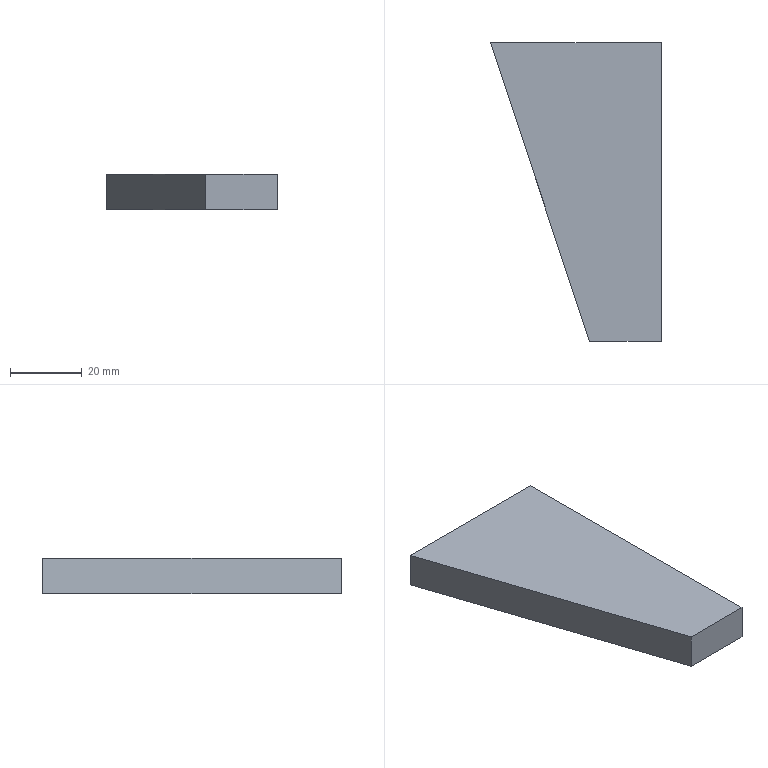Part | STEP file | 02-Reinforcing rib 13 | 1 solid | 6 faces | box 47.5 x 83 x 10 mm | volume 28013 mm3 | plane 6
STEP:
#1=CARTESIAN_POINT('',(0.,0.,0.));
#2=DIRECTION('',(0.,0.,1.));
#3=DIRECTION('',(1.,0.,0.));
#4=AXIS2_PLACEMENT_3D('',#1,#2,#3);
#5=CARTESIAN_POINT('',(0.,-83.,0.));
#6=VERTEX_POINT('',#5);
#7=CARTESIAN_POINT('',(0.,0.,0.));
#8=VERTEX_POINT('',#7);
#9=CARTESIAN_POINT('',(0.,0.,0.));
#10=DIRECTION('',(0.,1.,0.));
#11=VECTOR('',#10,1.);
#12=LINE('',#9,#11);
#13=CARTESIAN_POINT('',(0.,0.,10.));
#14=DIRECTION('',(-1.,0.,0.));
#15=DIRECTION('',(0.,-1.,0.));
#16=AXIS2_PLACEMENT_3D('',#13,#14,#15);
#17=PLANE('',#16);
#18=CARTESIAN_POINT('',(0.,-10.));
#19=DIRECTION('',(-1.,0.));
#20=VECTOR('',#19,1.);
#21=LINE('',#18,#20);
#22=(GEOMETRIC_REPRESENTATION_CONTEXT(2)PARAMETRIC_REPRESENTATION_CONTEXT()REPRESENTATION_CONTEXT('',''));
#23=DEFINITIONAL_REPRESENTATION('',(#21),#22);
#24=PCURVE('',#17,#23);
#25=CARTESIAN_POINT('',(0.,0.,0.));
#26=DIRECTION('',(0.,0.,-1.));
#27=DIRECTION('',(-1.,0.,0.));
#28=AXIS2_PLACEMENT_3D('',#25,#26,#27);
#29=PLANE('',#28);
#30=CARTESIAN_POINT('',(0.,0.));
#31=DIRECTION('',(0.,1.));
#32=VECTOR('',#31,1.);
#33=LINE('',#30,#32);
#34=(GEOMETRIC_REPRESENTATION_CONTEXT(2)PARAMETRIC_REPRESENTATION_CONTEXT()REPRESENTATION_CONTEXT('',''));
#35=DEFINITIONAL_REPRESENTATION('',(#33),#34);
#36=PCURVE('',#29,#35);
#37=SURFACE_CURVE('',#12,(#24,#36),.PCURVE_S1.);
#38=EDGE_CURVE('',#6,#8,#37,.T.);
#39=ORIENTED_EDGE('',*,*,#38,.T.);
#40=CARTESIAN_POINT('',(0.,0.,10.));
#41=VERTEX_POINT('',#40);
#42=CARTESIAN_POINT('',(0.,0.,10.));
#43=DIRECTION('',(0.,0.,-1.));
#44=VECTOR('',#43,1.);
#45=LINE('',#42,#44);
#46=CARTESIAN_POINT('',(0.,0.));
#47=DIRECTION('',(0.,-1.));
#48=VECTOR('',#47,1.);
#49=LINE('',#46,#48);
#50=(GEOMETRIC_REPRESENTATION_CONTEXT(2)PARAMETRIC_REPRESENTATION_CONTEXT()REPRESENTATION_CONTEXT('',''));
#51=DEFINITIONAL_REPRESENTATION('',(#49),#50);
#52=PCURVE('',#17,#51);
#53=CARTESIAN_POINT('',(0.,0.,10.));
#54=DIRECTION('',(0.,-1.,0.));
#55=DIRECTION('',(1.,0.,0.));
#56=AXIS2_PLACEMENT_3D('',#53,#54,#55);
#57=PLANE('',#56);
#58=CARTESIAN_POINT('',(0.,0.));
#59=DIRECTION('',(0.,-1.));
#60=VECTOR('',#59,1.);
#61=LINE('',#58,#60);
#62=(GEOMETRIC_REPRESENTATION_CONTEXT(2)PARAMETRIC_REPRESENTATION_CONTEXT()REPRESENTATION_CONTEXT('',''));
#63=DEFINITIONAL_REPRESENTATION('',(#61),#62);
#64=PCURVE('',#57,#63);
#65=SURFACE_CURVE('',#45,(#52,#64),.PCURVE_S1.);
#66=EDGE_CURVE('',#41,#8,#65,.T.);
#67=ORIENTED_EDGE('',*,*,#66,.F.);
#68=CARTESIAN_POINT('',(0.,-83.,10.));
#69=VERTEX_POINT('',#68);
#70=CARTESIAN_POINT('',(0.,0.,10.));
#71=DIRECTION('',(0.,1.,0.));
#72=VECTOR('',#71,1.);
#73=LINE('',#70,#72);
#74=CARTESIAN_POINT('',(0.,0.));
#75=DIRECTION('',(-1.,0.));
#76=VECTOR('',#75,1.);
#77=LINE('',#74,#76);
#78=(GEOMETRIC_REPRESENTATION_CONTEXT(2)PARAMETRIC_REPRESENTATION_CONTEXT()REPRESENTATION_CONTEXT('',''));
#79=DEFINITIONAL_REPRESENTATION('',(#77),#78);
#80=PCURVE('',#17,#79);
#81=CARTESIAN_POINT('',(0.,0.,10.));
#82=DIRECTION('',(0.,0.,-1.));
#83=DIRECTION('',(-1.,0.,0.));
#84=AXIS2_PLACEMENT_3D('',#81,#82,#83);
#85=PLANE('',#84);
#86=CARTESIAN_POINT('',(0.,0.));
#87=DIRECTION('',(0.,1.));
#88=VECTOR('',#87,1.);
#89=LINE('',#86,#88);
#90=(GEOMETRIC_REPRESENTATION_CONTEXT(2)PARAMETRIC_REPRESENTATION_CONTEXT()REPRESENTATION_CONTEXT('',''));
#91=DEFINITIONAL_REPRESENTATION('',(#89),#90);
#92=PCURVE('',#85,#91);
#93=SURFACE_CURVE('',#73,(#80,#92),.PCURVE_S1.);
#94=EDGE_CURVE('',#69,#41,#93,.T.);
#95=ORIENTED_EDGE('',*,*,#94,.F.);
#96=CARTESIAN_POINT('',(0.,-83.,10.));
#97=DIRECTION('',(0.,0.,-1.));
#98=VECTOR('',#97,1.);
#99=LINE('',#96,#98);
#100=CARTESIAN_POINT('',(83.,0.));
#101=DIRECTION('',(0.,-1.));
#102=VECTOR('',#101,1.);
#103=LINE('',#100,#102);
#104=(GEOMETRIC_REPRESENTATION_CONTEXT(2)PARAMETRIC_REPRESENTATION_CONTEXT()REPRESENTATION_CONTEXT('',''));
#105=DEFINITIONAL_REPRESENTATION('',(#103),#104);
#106=PCURVE('',#17,#105);
#107=CARTESIAN_POINT('',(0.,-83.,10.));
#108=DIRECTION('',(0.,1.,0.));
#109=DIRECTION('',(0.,0.,1.));
#110=AXIS2_PLACEMENT_3D('',#107,#108,#109);
#111=PLANE('',#110);
#112=CARTESIAN_POINT('',(0.,0.));
#113=DIRECTION('',(-1.,0.));
#114=VECTOR('',#113,1.);
#115=LINE('',#112,#114);
#116=(GEOMETRIC_REPRESENTATION_CONTEXT(2)PARAMETRIC_REPRESENTATION_CONTEXT()REPRESENTATION_CONTEXT('',''));
#117=DEFINITIONAL_REPRESENTATION('',(#115),#116);
#118=PCURVE('',#111,#117);
#119=SURFACE_CURVE('',#99,(#106,#118),.PCURVE_S1.);
#120=EDGE_CURVE('',#69,#6,#119,.T.);
#121=ORIENTED_EDGE('',*,*,#120,.T.);
#122=EDGE_LOOP('',(#39,#67,#95,#121));
#123=FACE_BOUND('',#122,.T.);
#124=ADVANCED_FACE('',(#123),#17,.F.);
#125=CARTESIAN_POINT('',(-47.5,0.,0.));
#126=VERTEX_POINT('',#125);
#127=CARTESIAN_POINT('',(0.,0.,0.));
#128=DIRECTION('',(-1.,0.,0.));
#129=VECTOR('',#128,1.);
#130=LINE('',#127,#129);
#131=CARTESIAN_POINT('',(0.,-10.));
#132=DIRECTION('',(-1.,0.));
#133=VECTOR('',#132,1.);
#134=LINE('',#131,#133);
#135=(GEOMETRIC_REPRESENTATION_CONTEXT(2)PARAMETRIC_REPRESENTATION_CONTEXT()REPRESENTATION_CONTEXT('',''));
#136=DEFINITIONAL_REPRESENTATION('',(#134),#135);
#137=PCURVE('',#57,#136);
#138=CARTESIAN_POINT('',(0.,0.));
#139=DIRECTION('',(1.,0.));
#140=VECTOR('',#139,1.);
#141=LINE('',#138,#140);
#142=(GEOMETRIC_REPRESENTATION_CONTEXT(2)PARAMETRIC_REPRESENTATION_CONTEXT()REPRESENTATION_CONTEXT('',''));
#143=DEFINITIONAL_REPRESENTATION('',(#141),#142);
#144=PCURVE('',#29,#143);
#145=SURFACE_CURVE('',#130,(#137,#144),.PCURVE_S1.);
#146=EDGE_CURVE('',#8,#126,#145,.T.);
#147=ORIENTED_EDGE('',*,*,#146,.T.);
#148=CARTESIAN_POINT('',(-47.5,0.,10.));
#149=VERTEX_POINT('',#148);
#150=CARTESIAN_POINT('',(-47.5,0.,10.));
#151=DIRECTION('',(0.,0.,-1.));
#152=VECTOR('',#151,1.);
#153=LINE('',#150,#152);
#154=CARTESIAN_POINT('',(-47.5,0.));
#155=DIRECTION('',(0.,-1.));
#156=VECTOR('',#155,1.);
#157=LINE('',#154,#156);
#158=(GEOMETRIC_REPRESENTATION_CONTEXT(2)PARAMETRIC_REPRESENTATION_CONTEXT()REPRESENTATION_CONTEXT('',''));
#159=DEFINITIONAL_REPRESENTATION('',(#157),#158);
#160=PCURVE('',#57,#159);
#161=CARTESIAN_POINT('',(-20.,-83.,10.));
#162=DIRECTION('',(0.9493,0.3145,0.));
#163=DIRECTION('',(-0.3145,0.9493,0.));
#164=AXIS2_PLACEMENT_3D('',#161,#162,#163);
#165=PLANE('',#164);
#166=CARTESIAN_POINT('',(87.437,0.));
#167=DIRECTION('',(0.,-1.));
#168=VECTOR('',#167,1.);
#169=LINE('',#166,#168);
#170=(GEOMETRIC_REPRESENTATION_CONTEXT(2)PARAMETRIC_REPRESENTATION_CONTEXT()REPRESENTATION_CONTEXT('',''));
#171=DEFINITIONAL_REPRESENTATION('',(#169),#170);
#172=PCURVE('',#165,#171);
#173=SURFACE_CURVE('',#153,(#160,#172),.PCURVE_S1.);
#174=EDGE_CURVE('',#149,#126,#173,.T.);
#175=ORIENTED_EDGE('',*,*,#174,.F.);
#176=CARTESIAN_POINT('',(0.,0.,10.));
#177=DIRECTION('',(-1.,0.,0.));
#178=VECTOR('',#177,1.);
#179=LINE('',#176,#178);
#180=CARTESIAN_POINT('',(0.,0.));
#181=DIRECTION('',(-1.,0.));
#182=VECTOR('',#181,1.);
#183=LINE('',#180,#182);
#184=(GEOMETRIC_REPRESENTATION_CONTEXT(2)PARAMETRIC_REPRESENTATION_CONTEXT()REPRESENTATION_CONTEXT('',''));
#185=DEFINITIONAL_REPRESENTATION('',(#183),#184);
#186=PCURVE('',#57,#185);
#187=CARTESIAN_POINT('',(0.,0.));
#188=DIRECTION('',(1.,0.));
#189=VECTOR('',#188,1.);
#190=LINE('',#187,#189);
#191=(GEOMETRIC_REPRESENTATION_CONTEXT(2)PARAMETRIC_REPRESENTATION_CONTEXT()REPRESENTATION_CONTEXT('',''));
#192=DEFINITIONAL_REPRESENTATION('',(#190),#191);
#193=PCURVE('',#85,#192);
#194=SURFACE_CURVE('',#179,(#186,#193),.PCURVE_S1.);
#195=EDGE_CURVE('',#41,#149,#194,.T.);
#196=ORIENTED_EDGE('',*,*,#195,.F.);
#197=ORIENTED_EDGE('',*,*,#66,.T.);
#198=EDGE_LOOP('',(#147,#175,#196,#197));
#199=FACE_BOUND('',#198,.T.);
#200=ADVANCED_FACE('',(#199),#57,.F.);
#201=CARTESIAN_POINT('',(-20.,-83.,0.));
#202=VERTEX_POINT('',#201);
#203=CARTESIAN_POINT('',(-20.,-83.,0.));
#204=DIRECTION('',(0.3145,-0.9493,0.));
#205=VECTOR('',#204,1.);
#206=LINE('',#203,#205);
#207=CARTESIAN_POINT('',(0.,-10.));
#208=DIRECTION('',(-1.,0.));
#209=VECTOR('',#208,1.);
#210=LINE('',#207,#209);
#211=(GEOMETRIC_REPRESENTATION_CONTEXT(2)PARAMETRIC_REPRESENTATION_CONTEXT()REPRESENTATION_CONTEXT('',''));
#212=DEFINITIONAL_REPRESENTATION('',(#210),#211);
#213=PCURVE('',#165,#212);
#214=CARTESIAN_POINT('',(20.,-83.));
#215=DIRECTION('',(-0.3145,-0.9493));
#216=VECTOR('',#215,1.);
#217=LINE('',#214,#216);
#218=(GEOMETRIC_REPRESENTATION_CONTEXT(2)PARAMETRIC_REPRESENTATION_CONTEXT()REPRESENTATION_CONTEXT('',''));
#219=DEFINITIONAL_REPRESENTATION('',(#217),#218);
#220=PCURVE('',#29,#219);
#221=SURFACE_CURVE('',#206,(#213,#220),.PCURVE_S1.);
#222=EDGE_CURVE('',#126,#202,#221,.T.);
#223=ORIENTED_EDGE('',*,*,#222,.T.);
#224=CARTESIAN_POINT('',(-20.,-83.,10.));
#225=VERTEX_POINT('',#224);
#226=CARTESIAN_POINT('',(-20.,-83.,10.));
#227=DIRECTION('',(0.,0.,-1.));
#228=VECTOR('',#227,1.);
#229=LINE('',#226,#228);
#230=CARTESIAN_POINT('',(0.,0.));
#231=DIRECTION('',(0.,-1.));
#232=VECTOR('',#231,1.);
#233=LINE('',#230,#232);
#234=(GEOMETRIC_REPRESENTATION_CONTEXT(2)PARAMETRIC_REPRESENTATION_CONTEXT()REPRESENTATION_CONTEXT('',''));
#235=DEFINITIONAL_REPRESENTATION('',(#233),#234);
#236=PCURVE('',#165,#235);
#237=CARTESIAN_POINT('',(0.,-20.));
#238=DIRECTION('',(-1.,0.));
#239=VECTOR('',#238,1.);
#240=LINE('',#237,#239);
#241=(GEOMETRIC_REPRESENTATION_CONTEXT(2)PARAMETRIC_REPRESENTATION_CONTEXT()REPRESENTATION_CONTEXT('',''));
#242=DEFINITIONAL_REPRESENTATION('',(#240),#241);
#243=PCURVE('',#111,#242);
#244=SURFACE_CURVE('',#229,(#236,#243),.PCURVE_S1.);
#245=EDGE_CURVE('',#225,#202,#244,.T.);
#246=ORIENTED_EDGE('',*,*,#245,.F.);
#247=CARTESIAN_POINT('',(-20.,-83.,10.));
#248=DIRECTION('',(0.3145,-0.9493,0.));
#249=VECTOR('',#248,1.);
#250=LINE('',#247,#249);
#251=CARTESIAN_POINT('',(0.,0.));
#252=DIRECTION('',(-1.,0.));
#253=VECTOR('',#252,1.);
#254=LINE('',#251,#253);
#255=(GEOMETRIC_REPRESENTATION_CONTEXT(2)PARAMETRIC_REPRESENTATION_CONTEXT()REPRESENTATION_CONTEXT('',''));
#256=DEFINITIONAL_REPRESENTATION('',(#254),#255);
#257=PCURVE('',#165,#256);
#258=CARTESIAN_POINT('',(20.,-83.));
#259=DIRECTION('',(-0.3145,-0.9493));
#260=VECTOR('',#259,1.);
#261=LINE('',#258,#260);
#262=(GEOMETRIC_REPRESENTATION_CONTEXT(2)PARAMETRIC_REPRESENTATION_CONTEXT()REPRESENTATION_CONTEXT('',''));
#263=DEFINITIONAL_REPRESENTATION('',(#261),#262);
#264=PCURVE('',#85,#263);
#265=SURFACE_CURVE('',#250,(#257,#264),.PCURVE_S1.);
#266=EDGE_CURVE('',#149,#225,#265,.T.);
#267=ORIENTED_EDGE('',*,*,#266,.F.);
#268=ORIENTED_EDGE('',*,*,#174,.T.);
#269=EDGE_LOOP('',(#223,#246,#267,#268));
#270=FACE_BOUND('',#269,.T.);
#271=ADVANCED_FACE('',(#270),#165,.F.);
#272=CARTESIAN_POINT('',(0.,-83.,0.));
#273=DIRECTION('',(1.,0.,0.));
#274=VECTOR('',#273,1.);
#275=LINE('',#272,#274);
#276=CARTESIAN_POINT('',(-10.,0.));
#277=DIRECTION('',(0.,1.));
#278=VECTOR('',#277,1.);
#279=LINE('',#276,#278);
#280=(GEOMETRIC_REPRESENTATION_CONTEXT(2)PARAMETRIC_REPRESENTATION_CONTEXT()REPRESENTATION_CONTEXT('',''));
#281=DEFINITIONAL_REPRESENTATION('',(#279),#280);
#282=PCURVE('',#111,#281);
#283=CARTESIAN_POINT('',(0.,-83.));
#284=DIRECTION('',(-1.,0.));
#285=VECTOR('',#284,1.);
#286=LINE('',#283,#285);
#287=(GEOMETRIC_REPRESENTATION_CONTEXT(2)PARAMETRIC_REPRESENTATION_CONTEXT()REPRESENTATION_CONTEXT('',''));
#288=DEFINITIONAL_REPRESENTATION('',(#286),#287);
#289=PCURVE('',#29,#288);
#290=SURFACE_CURVE('',#275,(#282,#289),.PCURVE_S1.);
#291=EDGE_CURVE('',#202,#6,#290,.T.);
#292=ORIENTED_EDGE('',*,*,#291,.T.);
#293=ORIENTED_EDGE('',*,*,#120,.F.);
#294=CARTESIAN_POINT('',(0.,-83.,10.));
#295=DIRECTION('',(1.,0.,0.));
#296=VECTOR('',#295,1.);
#297=LINE('',#294,#296);
#298=CARTESIAN_POINT('',(0.,0.));
#299=DIRECTION('',(0.,1.));
#300=VECTOR('',#299,1.);
#301=LINE('',#298,#300);
#302=(GEOMETRIC_REPRESENTATION_CONTEXT(2)PARAMETRIC_REPRESENTATION_CONTEXT()REPRESENTATION_CONTEXT('',''));
#303=DEFINITIONAL_REPRESENTATION('',(#301),#302);
#304=PCURVE('',#111,#303);
#305=CARTESIAN_POINT('',(0.,-83.));
#306=DIRECTION('',(-1.,0.));
#307=VECTOR('',#306,1.);
#308=LINE('',#305,#307);
#309=(GEOMETRIC_REPRESENTATION_CONTEXT(2)PARAMETRIC_REPRESENTATION_CONTEXT()REPRESENTATION_CONTEXT('',''));
#310=DEFINITIONAL_REPRESENTATION('',(#308),#309);
#311=PCURVE('',#85,#310);
#312=SURFACE_CURVE('',#297,(#304,#311),.PCURVE_S1.);
#313=EDGE_CURVE('',#225,#69,#312,.T.);
#314=ORIENTED_EDGE('',*,*,#313,.F.);
#315=ORIENTED_EDGE('',*,*,#245,.T.);
#316=EDGE_LOOP('',(#292,#293,#314,#315));
#317=FACE_BOUND('',#316,.T.);
#318=ADVANCED_FACE('',(#317),#111,.F.);
#319=ORIENTED_EDGE('',*,*,#94,.T.);
#320=ORIENTED_EDGE('',*,*,#195,.T.);
#321=ORIENTED_EDGE('',*,*,#266,.T.);
#322=ORIENTED_EDGE('',*,*,#313,.T.);
#323=EDGE_LOOP('',(#319,#320,#321,#322));
#324=FACE_BOUND('',#323,.T.);
#325=ADVANCED_FACE('',(#324),#85,.F.);
#326=ORIENTED_EDGE('',*,*,#38,.F.);
#327=ORIENTED_EDGE('',*,*,#291,.F.);
#328=ORIENTED_EDGE('',*,*,#222,.F.);
#329=ORIENTED_EDGE('',*,*,#146,.F.);
#330=EDGE_LOOP('',(#326,#327,#328,#329));
#331=FACE_BOUND('',#330,.T.);
#332=ADVANCED_FACE('',(#331),#29,.T.);
#333=CLOSED_SHELL('',(#124,#200,#271,#318,#325,#332));
#334=MANIFOLD_SOLID_BREP('',#333);
#335=(LENGTH_UNIT()NAMED_UNIT(*)SI_UNIT(.MILLI.,.METRE.));
#336=UNCERTAINTY_MEASURE_WITH_UNIT(LENGTH_MEASURE(0.0000001),#335,'','');
#337=(NAMED_UNIT(*)PLANE_ANGLE_UNIT()SI_UNIT($,.RADIAN.));
#338=(NAMED_UNIT(*)SI_UNIT($,.STERADIAN.)SOLID_ANGLE_UNIT());
#339=(GEOMETRIC_REPRESENTATION_CONTEXT(3)GLOBAL_UNCERTAINTY_ASSIGNED_CONTEXT((#336))GLOBAL_UNIT_ASSIGNED_CONTEXT((#335,#337,#338))REPRESENTATION_CONTEXT('',''));
#340=ADVANCED_BREP_SHAPE_REPRESENTATION('',(#4,#334),#339);